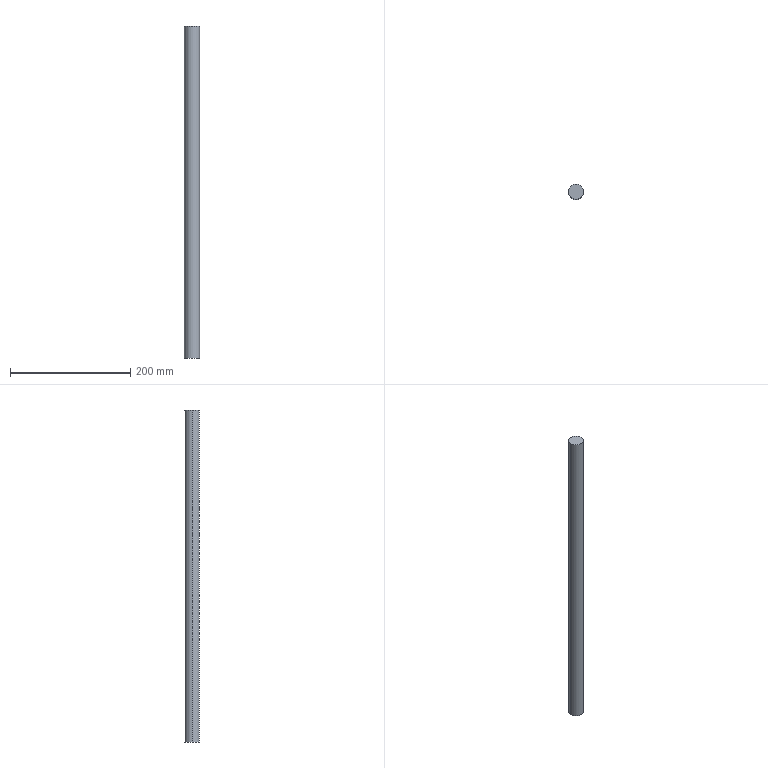Part | STEP file | Shaft dia 25 for small 31V11 | 1 solid | 4 faces | box 25 x 25 x 551.6 mm | volume 270766 mm3 | cylinder 2 | plane 2 | commonest cylinder face diameters 25 x2
STEP:
#1=CARTESIAN_POINT('',(0.,0.,0.));
#2=DIRECTION('',(0.,0.,1.));
#3=DIRECTION('',(1.,0.,0.));
#4=AXIS2_PLACEMENT_3D('',#1,#2,#3);
#5=CARTESIAN_POINT('',(12.5,0.,551.6));
#6=VERTEX_POINT('',#5);
#7=CARTESIAN_POINT('',(-12.5,0.,551.6));
#8=VERTEX_POINT('',#7);
#9=CARTESIAN_POINT('',(0.,0.,551.6));
#10=DIRECTION('',(0.,0.,1.));
#11=DIRECTION('',(1.,0.,0.));
#12=AXIS2_PLACEMENT_3D('',#9,#10,#11);
#13=CIRCLE('',#12,12.5);
#14=CARTESIAN_POINT('',(0.,0.,551.6));
#15=DIRECTION('',(0.,0.,-1.));
#16=DIRECTION('',(-1.,0.,0.));
#17=AXIS2_PLACEMENT_3D('',#14,#15,#16);
#18=CYLINDRICAL_SURFACE('',#17,12.5);
#19=CARTESIAN_POINT('',(3.142,0.));
#20=DIRECTION('',(-1.,0.));
#21=VECTOR('',#20,1.);
#22=LINE('',#19,#21);
#23=(GEOMETRIC_REPRESENTATION_CONTEXT(2)PARAMETRIC_REPRESENTATION_CONTEXT()REPRESENTATION_CONTEXT('',''));
#24=DEFINITIONAL_REPRESENTATION('',(#22),#23);
#25=PCURVE('',#18,#24);
#26=CARTESIAN_POINT('',(0.,0.,551.6));
#27=DIRECTION('',(0.,0.,1.));
#28=DIRECTION('',(1.,0.,0.));
#29=AXIS2_PLACEMENT_3D('',#26,#27,#28);
#30=PLANE('',#29);
#31=CARTESIAN_POINT('',(0.,0.));
#32=DIRECTION('',(1.,0.));
#33=AXIS2_PLACEMENT_2D('',#31,#32);
#34=CIRCLE('',#33,12.5);
#35=(GEOMETRIC_REPRESENTATION_CONTEXT(2)PARAMETRIC_REPRESENTATION_CONTEXT()REPRESENTATION_CONTEXT('',''));
#36=DEFINITIONAL_REPRESENTATION('',(#34),#35);
#37=PCURVE('',#30,#36);
#38=SURFACE_CURVE('',#13,(#25,#37),.PCURVE_S1.);
#39=EDGE_CURVE('',#6,#8,#38,.T.);
#40=ORIENTED_EDGE('',*,*,#39,.F.);
#41=CARTESIAN_POINT('',(12.5,0.,0.));
#42=VERTEX_POINT('',#41);
#43=CARTESIAN_POINT('',(12.5,0.,551.6));
#44=DIRECTION('',(0.,0.,-1.));
#45=VECTOR('',#44,1.);
#46=LINE('',#43,#45);
#47=CARTESIAN_POINT('',(3.142,0.));
#48=DIRECTION('',(0.,1.));
#49=VECTOR('',#48,1.);
#50=LINE('',#47,#49);
#51=(GEOMETRIC_REPRESENTATION_CONTEXT(2)PARAMETRIC_REPRESENTATION_CONTEXT()REPRESENTATION_CONTEXT('',''));
#52=DEFINITIONAL_REPRESENTATION('',(#50),#51);
#53=PCURVE('',#18,#52);
#54=CARTESIAN_POINT('',(0.,0.,551.6));
#55=DIRECTION('',(0.,0.,-1.));
#56=DIRECTION('',(-1.,0.,0.));
#57=AXIS2_PLACEMENT_3D('',#54,#55,#56);
#58=CYLINDRICAL_SURFACE('',#57,12.5);
#59=CARTESIAN_POINT('',(3.142,0.));
#60=DIRECTION('',(0.,1.));
#61=VECTOR('',#60,1.);
#62=LINE('',#59,#61);
#63=(GEOMETRIC_REPRESENTATION_CONTEXT(2)PARAMETRIC_REPRESENTATION_CONTEXT()REPRESENTATION_CONTEXT('',''));
#64=DEFINITIONAL_REPRESENTATION('',(#62),#63);
#65=PCURVE('',#58,#64);
#66=SURFACE_CURVE('',#46,(#53,#65),.PCURVE_S1.);
#67=EDGE_CURVE('',#6,#42,#66,.T.);
#68=ORIENTED_EDGE('',*,*,#67,.T.);
#69=CARTESIAN_POINT('',(-12.5,0.,0.));
#70=VERTEX_POINT('',#69);
#71=CARTESIAN_POINT('',(0.,0.,0.));
#72=DIRECTION('',(0.,0.,1.));
#73=DIRECTION('',(1.,0.,0.));
#74=AXIS2_PLACEMENT_3D('',#71,#72,#73);
#75=CIRCLE('',#74,12.5);
#76=CARTESIAN_POINT('',(3.142,551.6));
#77=DIRECTION('',(-1.,0.));
#78=VECTOR('',#77,1.);
#79=LINE('',#76,#78);
#80=(GEOMETRIC_REPRESENTATION_CONTEXT(2)PARAMETRIC_REPRESENTATION_CONTEXT()REPRESENTATION_CONTEXT('',''));
#81=DEFINITIONAL_REPRESENTATION('',(#79),#80);
#82=PCURVE('',#18,#81);
#83=CARTESIAN_POINT('',(0.,0.,0.));
#84=DIRECTION('',(0.,0.,1.));
#85=DIRECTION('',(1.,0.,0.));
#86=AXIS2_PLACEMENT_3D('',#83,#84,#85);
#87=PLANE('',#86);
#88=CARTESIAN_POINT('',(0.,0.));
#89=DIRECTION('',(1.,0.));
#90=AXIS2_PLACEMENT_2D('',#88,#89);
#91=CIRCLE('',#90,12.5);
#92=(GEOMETRIC_REPRESENTATION_CONTEXT(2)PARAMETRIC_REPRESENTATION_CONTEXT()REPRESENTATION_CONTEXT('',''));
#93=DEFINITIONAL_REPRESENTATION('',(#91),#92);
#94=PCURVE('',#87,#93);
#95=SURFACE_CURVE('',#75,(#82,#94),.PCURVE_S1.);
#96=EDGE_CURVE('',#42,#70,#95,.T.);
#97=ORIENTED_EDGE('',*,*,#96,.T.);
#98=CARTESIAN_POINT('',(-12.5,0.,551.6));
#99=DIRECTION('',(0.,0.,-1.));
#100=VECTOR('',#99,1.);
#101=LINE('',#98,#100);
#102=CARTESIAN_POINT('',(0.,0.));
#103=DIRECTION('',(0.,1.));
#104=VECTOR('',#103,1.);
#105=LINE('',#102,#104);
#106=(GEOMETRIC_REPRESENTATION_CONTEXT(2)PARAMETRIC_REPRESENTATION_CONTEXT()REPRESENTATION_CONTEXT('',''));
#107=DEFINITIONAL_REPRESENTATION('',(#105),#106);
#108=PCURVE('',#18,#107);
#109=CARTESIAN_POINT('',(6.283,0.));
#110=DIRECTION('',(0.,1.));
#111=VECTOR('',#110,1.);
#112=LINE('',#109,#111);
#113=(GEOMETRIC_REPRESENTATION_CONTEXT(2)PARAMETRIC_REPRESENTATION_CONTEXT()REPRESENTATION_CONTEXT('',''));
#114=DEFINITIONAL_REPRESENTATION('',(#112),#113);
#115=PCURVE('',#58,#114);
#116=SURFACE_CURVE('',#101,(#108,#115),.PCURVE_S1.);
#117=EDGE_CURVE('',#8,#70,#116,.T.);
#118=ORIENTED_EDGE('',*,*,#117,.F.);
#119=EDGE_LOOP('',(#40,#68,#97,#118));
#120=FACE_BOUND('',#119,.T.);
#121=ADVANCED_FACE('',(#120),#18,.T.);
#122=ORIENTED_EDGE('',*,*,#67,.F.);
#123=CARTESIAN_POINT('',(0.,0.,551.6));
#124=DIRECTION('',(0.,0.,1.));
#125=DIRECTION('',(1.,0.,0.));
#126=AXIS2_PLACEMENT_3D('',#123,#124,#125);
#127=CIRCLE('',#126,12.5);
#128=CARTESIAN_POINT('',(9.425,0.));
#129=DIRECTION('',(-1.,0.));
#130=VECTOR('',#129,1.);
#131=LINE('',#128,#130);
#132=(GEOMETRIC_REPRESENTATION_CONTEXT(2)PARAMETRIC_REPRESENTATION_CONTEXT()REPRESENTATION_CONTEXT('',''));
#133=DEFINITIONAL_REPRESENTATION('',(#131),#132);
#134=PCURVE('',#58,#133);
#135=CARTESIAN_POINT('',(0.,0.));
#136=DIRECTION('',(1.,0.));
#137=AXIS2_PLACEMENT_2D('',#135,#136);
#138=CIRCLE('',#137,12.5);
#139=(GEOMETRIC_REPRESENTATION_CONTEXT(2)PARAMETRIC_REPRESENTATION_CONTEXT()REPRESENTATION_CONTEXT('',''));
#140=DEFINITIONAL_REPRESENTATION('',(#138),#139);
#141=PCURVE('',#30,#140);
#142=SURFACE_CURVE('',#127,(#134,#141),.PCURVE_S1.);
#143=EDGE_CURVE('',#8,#6,#142,.T.);
#144=ORIENTED_EDGE('',*,*,#143,.F.);
#145=ORIENTED_EDGE('',*,*,#117,.T.);
#146=CARTESIAN_POINT('',(0.,0.,0.));
#147=DIRECTION('',(0.,0.,1.));
#148=DIRECTION('',(1.,0.,0.));
#149=AXIS2_PLACEMENT_3D('',#146,#147,#148);
#150=CIRCLE('',#149,12.5);
#151=CARTESIAN_POINT('',(9.425,551.6));
#152=DIRECTION('',(-1.,0.));
#153=VECTOR('',#152,1.);
#154=LINE('',#151,#153);
#155=(GEOMETRIC_REPRESENTATION_CONTEXT(2)PARAMETRIC_REPRESENTATION_CONTEXT()REPRESENTATION_CONTEXT('',''));
#156=DEFINITIONAL_REPRESENTATION('',(#154),#155);
#157=PCURVE('',#58,#156);
#158=CARTESIAN_POINT('',(0.,0.));
#159=DIRECTION('',(1.,0.));
#160=AXIS2_PLACEMENT_2D('',#158,#159);
#161=CIRCLE('',#160,12.5);
#162=(GEOMETRIC_REPRESENTATION_CONTEXT(2)PARAMETRIC_REPRESENTATION_CONTEXT()REPRESENTATION_CONTEXT('',''));
#163=DEFINITIONAL_REPRESENTATION('',(#161),#162);
#164=PCURVE('',#87,#163);
#165=SURFACE_CURVE('',#150,(#157,#164),.PCURVE_S1.);
#166=EDGE_CURVE('',#70,#42,#165,.T.);
#167=ORIENTED_EDGE('',*,*,#166,.T.);
#168=EDGE_LOOP('',(#122,#144,#145,#167));
#169=FACE_BOUND('',#168,.T.);
#170=ADVANCED_FACE('',(#169),#58,.T.);
#171=ORIENTED_EDGE('',*,*,#143,.T.);
#172=ORIENTED_EDGE('',*,*,#39,.T.);
#173=EDGE_LOOP('',(#171,#172));
#174=FACE_BOUND('',#173,.T.);
#175=ADVANCED_FACE('',(#174),#30,.T.);
#176=ORIENTED_EDGE('',*,*,#166,.F.);
#177=ORIENTED_EDGE('',*,*,#96,.F.);
#178=EDGE_LOOP('',(#176,#177));
#179=FACE_BOUND('',#178,.T.);
#180=ADVANCED_FACE('',(#179),#87,.F.);
#181=CLOSED_SHELL('',(#121,#170,#175,#180));
#182=MANIFOLD_SOLID_BREP('',#181);
#183=(LENGTH_UNIT()NAMED_UNIT(*)SI_UNIT(.MILLI.,.METRE.));
#184=UNCERTAINTY_MEASURE_WITH_UNIT(LENGTH_MEASURE(0.0000001),#183,'','');
#185=(NAMED_UNIT(*)PLANE_ANGLE_UNIT()SI_UNIT($,.RADIAN.));
#186=(NAMED_UNIT(*)SI_UNIT($,.STERADIAN.)SOLID_ANGLE_UNIT());
#187=(GEOMETRIC_REPRESENTATION_CONTEXT(3)GLOBAL_UNCERTAINTY_ASSIGNED_CONTEXT((#184))GLOBAL_UNIT_ASSIGNED_CONTEXT((#183,#185,#186))REPRESENTATION_CONTEXT('',''));
#188=ADVANCED_BREP_SHAPE_REPRESENTATION('',(#4,#182),#187);